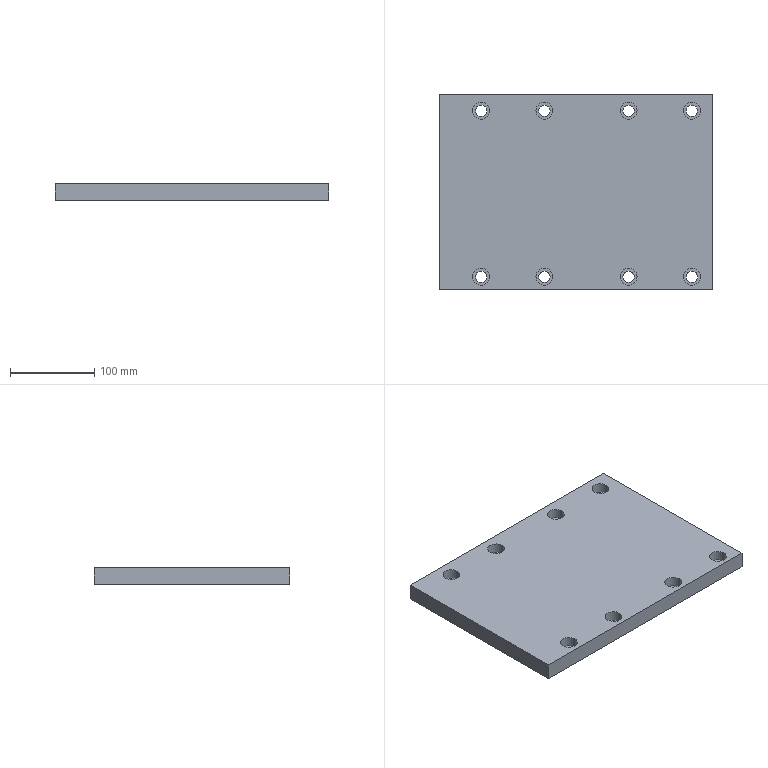Part | SolidWorks | features BaseBody 1 | 1 solid | 46 faces | box 325 x 232 x 20 mm | volume 1468680 mm3 | cylinder 32 | plane 14 | commonest cylinder face diameters 13.5 x16 20 x16
STEP:
#1=CARTESIAN_POINT('',(-122.5,96.448,8.));
#2=VERTEX_POINT('',#1);
#3=CARTESIAN_POINT('',(-102.5,96.448,8.));
#4=VERTEX_POINT('',#3);
#5=CARTESIAN_POINT('',(-112.5,96.448,8.));
#6=DIRECTION('',(0.,0.,1.));
#7=DIRECTION('',(1.,0.,0.));
#8=AXIS2_PLACEMENT_3D('',#5,#6,#7);
#9=CIRCLE('',#8,10.);
#10=EDGE_CURVE('',#2,#4,#9,.T.);
#11=ORIENTED_EDGE('',*,*,#10,.F.);
#12=CARTESIAN_POINT('',(-122.5,96.448,20.));
#13=VERTEX_POINT('',#12);
#14=CARTESIAN_POINT('',(-122.5,96.448,20.));
#15=DIRECTION('',(0.,0.,1.));
#16=VECTOR('',#15,1000.);
#17=LINE('',#14,#16);
#18=EDGE_CURVE('',#2,#13,#17,.T.);
#19=ORIENTED_EDGE('',*,*,#18,.T.);
#20=CARTESIAN_POINT('',(-102.5,96.448,20.));
#21=VERTEX_POINT('',#20);
#22=CARTESIAN_POINT('',(-112.5,96.448,20.));
#23=DIRECTION('',(0.,0.,1.));
#24=DIRECTION('',(1.,0.,0.));
#25=AXIS2_PLACEMENT_3D('',#22,#23,#24);
#26=CIRCLE('',#25,10.);
#27=EDGE_CURVE('',#13,#21,#26,.T.);
#28=ORIENTED_EDGE('',*,*,#27,.T.);
#29=CARTESIAN_POINT('',(-102.5,96.448,20.));
#30=DIRECTION('',(0.,0.,1.));
#31=VECTOR('',#30,1000.);
#32=LINE('',#29,#31);
#33=EDGE_CURVE('',#4,#21,#32,.T.);
#34=ORIENTED_EDGE('',*,*,#33,.F.);
#35=EDGE_LOOP('',(#11,#19,#28,#34));
#36=FACE_OUTER_BOUND('',#35,.T.);
#37=CARTESIAN_POINT('',(-112.5,96.448,20.));
#38=DIRECTION('',(0.,0.,1.));
#39=DIRECTION('',(1.,0.,0.));
#40=AXIS2_PLACEMENT_3D('',#37,#38,#39);
#41=CYLINDRICAL_SURFACE('',#40,10.);
#42=ADVANCED_FACE('',(#36),#41,.F.);
#43=CARTESIAN_POINT('',(-119.25,96.448,0.));
#44=VERTEX_POINT('',#43);
#45=CARTESIAN_POINT('',(-105.75,96.448,0.));
#46=VERTEX_POINT('',#45);
#47=CARTESIAN_POINT('',(-112.5,96.448,0.));
#48=DIRECTION('',(0.,0.,1.));
#49=DIRECTION('',(1.,0.,0.));
#50=AXIS2_PLACEMENT_3D('',#47,#48,#49);
#51=CIRCLE('',#50,6.75);
#52=EDGE_CURVE('',#44,#46,#51,.T.);
#53=ORIENTED_EDGE('',*,*,#52,.F.);
#54=CARTESIAN_POINT('',(-119.25,96.448,8.));
#55=VERTEX_POINT('',#54);
#56=CARTESIAN_POINT('',(-119.25,96.448,20.));
#57=DIRECTION('',(0.,0.,1.));
#58=VECTOR('',#57,1000.);
#59=LINE('',#56,#58);
#60=EDGE_CURVE('',#44,#55,#59,.T.);
#61=ORIENTED_EDGE('',*,*,#60,.T.);
#62=CARTESIAN_POINT('',(-105.75,96.448,8.));
#63=VERTEX_POINT('',#62);
#64=CARTESIAN_POINT('',(-112.5,96.448,8.));
#65=DIRECTION('',(0.,0.,1.));
#66=DIRECTION('',(1.,0.,0.));
#67=AXIS2_PLACEMENT_3D('',#64,#65,#66);
#68=CIRCLE('',#67,6.75);
#69=EDGE_CURVE('',#55,#63,#68,.T.);
#70=ORIENTED_EDGE('',*,*,#69,.T.);
#71=CARTESIAN_POINT('',(-105.75,96.448,20.));
#72=DIRECTION('',(0.,0.,1.));
#73=VECTOR('',#72,1000.);
#74=LINE('',#71,#73);
#75=EDGE_CURVE('',#46,#63,#74,.T.);
#76=ORIENTED_EDGE('',*,*,#75,.F.);
#77=EDGE_LOOP('',(#53,#61,#70,#76));
#78=FACE_OUTER_BOUND('',#77,.T.);
#79=CARTESIAN_POINT('',(-112.5,96.448,20.));
#80=DIRECTION('',(0.,0.,1.));
#81=DIRECTION('',(1.,0.,0.));
#82=AXIS2_PLACEMENT_3D('',#79,#80,#81);
#83=CYLINDRICAL_SURFACE('',#82,6.75);
#84=ADVANCED_FACE('',(#78),#83,.F.);
#85=CARTESIAN_POINT('',(-47.5,96.448,8.));
#86=VERTEX_POINT('',#85);
#87=CARTESIAN_POINT('',(-27.5,96.448,8.));
#88=VERTEX_POINT('',#87);
#89=CARTESIAN_POINT('',(-37.5,96.448,8.));
#90=DIRECTION('',(0.,0.,1.));
#91=DIRECTION('',(1.,0.,0.));
#92=AXIS2_PLACEMENT_3D('',#89,#90,#91);
#93=CIRCLE('',#92,10.);
#94=EDGE_CURVE('',#86,#88,#93,.T.);
#95=ORIENTED_EDGE('',*,*,#94,.F.);
#96=CARTESIAN_POINT('',(-47.5,96.448,20.));
#97=VERTEX_POINT('',#96);
#98=CARTESIAN_POINT('',(-47.5,96.448,20.));
#99=DIRECTION('',(0.,0.,1.));
#100=VECTOR('',#99,1000.);
#101=LINE('',#98,#100);
#102=EDGE_CURVE('',#86,#97,#101,.T.);
#103=ORIENTED_EDGE('',*,*,#102,.T.);
#104=CARTESIAN_POINT('',(-27.5,96.448,20.));
#105=VERTEX_POINT('',#104);
#106=CARTESIAN_POINT('',(-37.5,96.448,20.));
#107=DIRECTION('',(0.,0.,1.));
#108=DIRECTION('',(1.,0.,0.));
#109=AXIS2_PLACEMENT_3D('',#106,#107,#108);
#110=CIRCLE('',#109,10.);
#111=EDGE_CURVE('',#97,#105,#110,.T.);
#112=ORIENTED_EDGE('',*,*,#111,.T.);
#113=CARTESIAN_POINT('',(-27.5,96.448,20.));
#114=DIRECTION('',(0.,0.,1.));
#115=VECTOR('',#114,1000.);
#116=LINE('',#113,#115);
#117=EDGE_CURVE('',#88,#105,#116,.T.);
#118=ORIENTED_EDGE('',*,*,#117,.F.);
#119=EDGE_LOOP('',(#95,#103,#112,#118));
#120=FACE_OUTER_BOUND('',#119,.T.);
#121=CARTESIAN_POINT('',(-37.5,96.448,20.));
#122=DIRECTION('',(0.,0.,1.));
#123=DIRECTION('',(1.,0.,0.));
#124=AXIS2_PLACEMENT_3D('',#121,#122,#123);
#125=CYLINDRICAL_SURFACE('',#124,10.);
#126=ADVANCED_FACE('',(#120),#125,.F.);
#127=CARTESIAN_POINT('',(-44.25,96.448,0.));
#128=VERTEX_POINT('',#127);
#129=CARTESIAN_POINT('',(-30.75,96.448,0.));
#130=VERTEX_POINT('',#129);
#131=CARTESIAN_POINT('',(-37.5,96.448,0.));
#132=DIRECTION('',(0.,0.,1.));
#133=DIRECTION('',(1.,0.,0.));
#134=AXIS2_PLACEMENT_3D('',#131,#132,#133);
#135=CIRCLE('',#134,6.75);
#136=EDGE_CURVE('',#128,#130,#135,.T.);
#137=ORIENTED_EDGE('',*,*,#136,.F.);
#138=CARTESIAN_POINT('',(-44.25,96.448,8.));
#139=VERTEX_POINT('',#138);
#140=CARTESIAN_POINT('',(-44.25,96.448,20.));
#141=DIRECTION('',(0.,0.,1.));
#142=VECTOR('',#141,1000.);
#143=LINE('',#140,#142);
#144=EDGE_CURVE('',#128,#139,#143,.T.);
#145=ORIENTED_EDGE('',*,*,#144,.T.);
#146=CARTESIAN_POINT('',(-30.75,96.448,8.));
#147=VERTEX_POINT('',#146);
#148=CARTESIAN_POINT('',(-37.5,96.448,8.));
#149=DIRECTION('',(0.,0.,1.));
#150=DIRECTION('',(1.,0.,0.));
#151=AXIS2_PLACEMENT_3D('',#148,#149,#150);
#152=CIRCLE('',#151,6.75);
#153=EDGE_CURVE('',#139,#147,#152,.T.);
#154=ORIENTED_EDGE('',*,*,#153,.T.);
#155=CARTESIAN_POINT('',(-30.75,96.448,20.));
#156=DIRECTION('',(0.,0.,1.));
#157=VECTOR('',#156,1000.);
#158=LINE('',#155,#157);
#159=EDGE_CURVE('',#130,#147,#158,.T.);
#160=ORIENTED_EDGE('',*,*,#159,.F.);
#161=EDGE_LOOP('',(#137,#145,#154,#160));
#162=FACE_OUTER_BOUND('',#161,.T.);
#163=CARTESIAN_POINT('',(-37.5,96.448,20.));
#164=DIRECTION('',(0.,0.,1.));
#165=DIRECTION('',(1.,0.,0.));
#166=AXIS2_PLACEMENT_3D('',#163,#164,#165);
#167=CYLINDRICAL_SURFACE('',#166,6.75);
#168=ADVANCED_FACE('',(#162),#167,.F.);
#169=CARTESIAN_POINT('',(52.5,96.448,8.));
#170=VERTEX_POINT('',#169);
#171=CARTESIAN_POINT('',(72.5,96.448,8.));
#172=VERTEX_POINT('',#171);
#173=CARTESIAN_POINT('',(62.5,96.448,8.));
#174=DIRECTION('',(0.,0.,1.));
#175=DIRECTION('',(1.,0.,0.));
#176=AXIS2_PLACEMENT_3D('',#173,#174,#175);
#177=CIRCLE('',#176,10.);
#178=EDGE_CURVE('',#170,#172,#177,.T.);
#179=ORIENTED_EDGE('',*,*,#178,.F.);
#180=CARTESIAN_POINT('',(52.5,96.448,20.));
#181=VERTEX_POINT('',#180);
#182=CARTESIAN_POINT('',(52.5,96.448,20.));
#183=DIRECTION('',(0.,0.,1.));
#184=VECTOR('',#183,1000.);
#185=LINE('',#182,#184);
#186=EDGE_CURVE('',#170,#181,#185,.T.);
#187=ORIENTED_EDGE('',*,*,#186,.T.);
#188=CARTESIAN_POINT('',(72.5,96.448,20.));
#189=VERTEX_POINT('',#188);
#190=CARTESIAN_POINT('',(62.5,96.448,20.));
#191=DIRECTION('',(0.,0.,1.));
#192=DIRECTION('',(1.,0.,0.));
#193=AXIS2_PLACEMENT_3D('',#190,#191,#192);
#194=CIRCLE('',#193,10.);
#195=EDGE_CURVE('',#181,#189,#194,.T.);
#196=ORIENTED_EDGE('',*,*,#195,.T.);
#197=CARTESIAN_POINT('',(72.5,96.448,20.));
#198=DIRECTION('',(0.,0.,1.));
#199=VECTOR('',#198,1000.);
#200=LINE('',#197,#199);
#201=EDGE_CURVE('',#172,#189,#200,.T.);
#202=ORIENTED_EDGE('',*,*,#201,.F.);
#203=EDGE_LOOP('',(#179,#187,#196,#202));
#204=FACE_OUTER_BOUND('',#203,.T.);
#205=CARTESIAN_POINT('',(62.5,96.448,20.));
#206=DIRECTION('',(0.,0.,1.));
#207=DIRECTION('',(1.,0.,0.));
#208=AXIS2_PLACEMENT_3D('',#205,#206,#207);
#209=CYLINDRICAL_SURFACE('',#208,10.);
#210=ADVANCED_FACE('',(#204),#209,.F.);
#211=CARTESIAN_POINT('',(55.75,96.448,0.));
#212=VERTEX_POINT('',#211);
#213=CARTESIAN_POINT('',(69.25,96.448,0.));
#214=VERTEX_POINT('',#213);
#215=CARTESIAN_POINT('',(62.5,96.448,0.));
#216=DIRECTION('',(0.,0.,1.));
#217=DIRECTION('',(1.,0.,0.));
#218=AXIS2_PLACEMENT_3D('',#215,#216,#217);
#219=CIRCLE('',#218,6.75);
#220=EDGE_CURVE('',#212,#214,#219,.T.);
#221=ORIENTED_EDGE('',*,*,#220,.F.);
#222=CARTESIAN_POINT('',(55.75,96.448,8.));
#223=VERTEX_POINT('',#222);
#224=CARTESIAN_POINT('',(55.75,96.448,20.));
#225=DIRECTION('',(0.,0.,1.));
#226=VECTOR('',#225,1000.);
#227=LINE('',#224,#226);
#228=EDGE_CURVE('',#212,#223,#227,.T.);
#229=ORIENTED_EDGE('',*,*,#228,.T.);
#230=CARTESIAN_POINT('',(69.25,96.448,8.));
#231=VERTEX_POINT('',#230);
#232=CARTESIAN_POINT('',(62.5,96.448,8.));
#233=DIRECTION('',(0.,0.,1.));
#234=DIRECTION('',(1.,0.,0.));
#235=AXIS2_PLACEMENT_3D('',#232,#233,#234);
#236=CIRCLE('',#235,6.75);
#237=EDGE_CURVE('',#223,#231,#236,.T.);
#238=ORIENTED_EDGE('',*,*,#237,.T.);
#239=CARTESIAN_POINT('',(69.25,96.448,20.));
#240=DIRECTION('',(0.,0.,1.));
#241=VECTOR('',#240,1000.);
#242=LINE('',#239,#241);
#243=EDGE_CURVE('',#214,#231,#242,.T.);
#244=ORIENTED_EDGE('',*,*,#243,.F.);
#245=EDGE_LOOP('',(#221,#229,#238,#244));
#246=FACE_OUTER_BOUND('',#245,.T.);
#247=CARTESIAN_POINT('',(62.5,96.448,20.));
#248=DIRECTION('',(0.,0.,1.));
#249=DIRECTION('',(1.,0.,0.));
#250=AXIS2_PLACEMENT_3D('',#247,#248,#249);
#251=CYLINDRICAL_SURFACE('',#250,6.75);
#252=ADVANCED_FACE('',(#246),#251,.F.);
#253=CARTESIAN_POINT('',(127.5,96.448,8.));
#254=VERTEX_POINT('',#253);
#255=CARTESIAN_POINT('',(147.5,96.448,8.));
#256=VERTEX_POINT('',#255);
#257=CARTESIAN_POINT('',(137.5,96.448,8.));
#258=DIRECTION('',(0.,0.,1.));
#259=DIRECTION('',(1.,0.,0.));
#260=AXIS2_PLACEMENT_3D('',#257,#258,#259);
#261=CIRCLE('',#260,10.);
#262=EDGE_CURVE('',#254,#256,#261,.T.);
#263=ORIENTED_EDGE('',*,*,#262,.F.);
#264=CARTESIAN_POINT('',(127.5,96.448,20.));
#265=VERTEX_POINT('',#264);
#266=CARTESIAN_POINT('',(127.5,96.448,20.));
#267=DIRECTION('',(0.,0.,1.));
#268=VECTOR('',#267,1000.);
#269=LINE('',#266,#268);
#270=EDGE_CURVE('',#254,#265,#269,.T.);
#271=ORIENTED_EDGE('',*,*,#270,.T.);
#272=CARTESIAN_POINT('',(147.5,96.448,20.));
#273=VERTEX_POINT('',#272);
#274=CARTESIAN_POINT('',(137.5,96.448,20.));
#275=DIRECTION('',(0.,0.,1.));
#276=DIRECTION('',(1.,0.,0.));
#277=AXIS2_PLACEMENT_3D('',#274,#275,#276);
#278=CIRCLE('',#277,10.);
#279=EDGE_CURVE('',#265,#273,#278,.T.);
#280=ORIENTED_EDGE('',*,*,#279,.T.);
#281=CARTESIAN_POINT('',(147.5,96.448,20.));
#282=DIRECTION('',(0.,0.,1.));
#283=VECTOR('',#282,1000.);
#284=LINE('',#281,#283);
#285=EDGE_CURVE('',#256,#273,#284,.T.);
#286=ORIENTED_EDGE('',*,*,#285,.F.);
#287=EDGE_LOOP('',(#263,#271,#280,#286));
#288=FACE_OUTER_BOUND('',#287,.T.);
#289=CARTESIAN_POINT('',(137.5,96.448,20.));
#290=DIRECTION('',(0.,0.,1.));
#291=DIRECTION('',(1.,0.,0.));
#292=AXIS2_PLACEMENT_3D('',#289,#290,#291);
#293=CYLINDRICAL_SURFACE('',#292,10.);
#294=ADVANCED_FACE('',(#288),#293,.F.);
#295=CARTESIAN_POINT('',(130.75,96.448,0.));
#296=VERTEX_POINT('',#295);
#297=CARTESIAN_POINT('',(144.25,96.448,0.));
#298=VERTEX_POINT('',#297);
#299=CARTESIAN_POINT('',(137.5,96.448,0.));
#300=DIRECTION('',(0.,0.,1.));
#301=DIRECTION('',(1.,0.,0.));
#302=AXIS2_PLACEMENT_3D('',#299,#300,#301);
#303=CIRCLE('',#302,6.75);
#304=EDGE_CURVE('',#296,#298,#303,.T.);
#305=ORIENTED_EDGE('',*,*,#304,.F.);
#306=CARTESIAN_POINT('',(130.75,96.448,8.));
#307=VERTEX_POINT('',#306);
#308=CARTESIAN_POINT('',(130.75,96.448,20.));
#309=DIRECTION('',(0.,0.,1.));
#310=VECTOR('',#309,1000.);
#311=LINE('',#308,#310);
#312=EDGE_CURVE('',#296,#307,#311,.T.);
#313=ORIENTED_EDGE('',*,*,#312,.T.);
#314=CARTESIAN_POINT('',(144.25,96.448,8.));
#315=VERTEX_POINT('',#314);
#316=CARTESIAN_POINT('',(137.5,96.448,8.));
#317=DIRECTION('',(0.,0.,1.));
#318=DIRECTION('',(1.,0.,0.));
#319=AXIS2_PLACEMENT_3D('',#316,#317,#318);
#320=CIRCLE('',#319,6.75);
#321=EDGE_CURVE('',#307,#315,#320,.T.);
#322=ORIENTED_EDGE('',*,*,#321,.T.);
#323=CARTESIAN_POINT('',(144.25,96.448,20.));
#324=DIRECTION('',(0.,0.,1.));
#325=VECTOR('',#324,1000.);
#326=LINE('',#323,#325);
#327=EDGE_CURVE('',#298,#315,#326,.T.);
#328=ORIENTED_EDGE('',*,*,#327,.F.);
#329=EDGE_LOOP('',(#305,#313,#322,#328));
#330=FACE_OUTER_BOUND('',#329,.T.);
#331=CARTESIAN_POINT('',(137.5,96.448,20.));
#332=DIRECTION('',(0.,0.,1.));
#333=DIRECTION('',(1.,0.,0.));
#334=AXIS2_PLACEMENT_3D('',#331,#332,#333);
#335=CYLINDRICAL_SURFACE('',#334,6.75);
#336=ADVANCED_FACE('',(#330),#335,.F.);
#337=CARTESIAN_POINT('',(127.5,-100.552,8.));
#338=VERTEX_POINT('',#337);
#339=CARTESIAN_POINT('',(147.5,-100.552,8.));
#340=VERTEX_POINT('',#339);
#341=CARTESIAN_POINT('',(137.5,-100.552,8.));
#342=DIRECTION('',(0.,0.,1.));
#343=DIRECTION('',(1.,0.,0.));
#344=AXIS2_PLACEMENT_3D('',#341,#342,#343);
#345=CIRCLE('',#344,10.);
#346=EDGE_CURVE('',#338,#340,#345,.T.);
#347=ORIENTED_EDGE('',*,*,#346,.F.);
#348=CARTESIAN_POINT('',(127.5,-100.552,20.));
#349=VERTEX_POINT('',#348);
#350=CARTESIAN_POINT('',(127.5,-100.552,20.));
#351=DIRECTION('',(0.,0.,1.));
#352=VECTOR('',#351,1000.);
#353=LINE('',#350,#352);
#354=EDGE_CURVE('',#338,#349,#353,.T.);
#355=ORIENTED_EDGE('',*,*,#354,.T.);
#356=CARTESIAN_POINT('',(147.5,-100.552,20.));
#357=VERTEX_POINT('',#356);
#358=CARTESIAN_POINT('',(137.5,-100.552,20.));
#359=DIRECTION('',(0.,0.,1.));
#360=DIRECTION('',(1.,0.,0.));
#361=AXIS2_PLACEMENT_3D('',#358,#359,#360);
#362=CIRCLE('',#361,10.);
#363=EDGE_CURVE('',#349,#357,#362,.T.);
#364=ORIENTED_EDGE('',*,*,#363,.T.);
#365=CARTESIAN_POINT('',(147.5,-100.552,20.));
#366=DIRECTION('',(0.,0.,1.));
#367=VECTOR('',#366,1000.);
#368=LINE('',#365,#367);
#369=EDGE_CURVE('',#340,#357,#368,.T.);
#370=ORIENTED_EDGE('',*,*,#369,.F.);
#371=EDGE_LOOP('',(#347,#355,#364,#370));
#372=FACE_OUTER_BOUND('',#371,.T.);
#373=CARTESIAN_POINT('',(137.5,-100.552,20.));
#374=DIRECTION('',(0.,0.,1.));
#375=DIRECTION('',(1.,0.,0.));
#376=AXIS2_PLACEMENT_3D('',#373,#374,#375);
#377=CYLINDRICAL_SURFACE('',#376,10.);
#378=ADVANCED_FACE('',(#372),#377,.F.);
#379=CARTESIAN_POINT('',(130.75,-100.552,0.));
#380=VERTEX_POINT('',#379);
#381=CARTESIAN_POINT('',(144.25,-100.552,0.));
#382=VERTEX_POINT('',#381);
#383=CARTESIAN_POINT('',(137.5,-100.552,0.));
#384=DIRECTION('',(0.,0.,1.));
#385=DIRECTION('',(1.,0.,0.));
#386=AXIS2_PLACEMENT_3D('',#383,#384,#385);
#387=CIRCLE('',#386,6.75);
#388=EDGE_CURVE('',#380,#382,#387,.T.);
#389=ORIENTED_EDGE('',*,*,#388,.F.);
#390=CARTESIAN_POINT('',(130.75,-100.552,8.));
#391=VERTEX_POINT('',#390);
#392=CARTESIAN_POINT('',(130.75,-100.552,20.));
#393=DIRECTION('',(0.,0.,1.));
#394=VECTOR('',#393,1000.);
#395=LINE('',#392,#394);
#396=EDGE_CURVE('',#380,#391,#395,.T.);
#397=ORIENTED_EDGE('',*,*,#396,.T.);
#398=CARTESIAN_POINT('',(144.25,-100.552,8.));
#399=VERTEX_POINT('',#398);
#400=CARTESIAN_POINT('',(137.5,-100.552,8.));
#401=DIRECTION('',(0.,0.,1.));
#402=DIRECTION('',(1.,0.,0.));
#403=AXIS2_PLACEMENT_3D('',#400,#401,#402);
#404=CIRCLE('',#403,6.75);
#405=EDGE_CURVE('',#391,#399,#404,.T.);
#406=ORIENTED_EDGE('',*,*,#405,.T.);
#407=CARTESIAN_POINT('',(144.25,-100.552,20.));
#408=DIRECTION('',(0.,0.,1.));
#409=VECTOR('',#408,1000.);
#410=LINE('',#407,#409);
#411=EDGE_CURVE('',#382,#399,#410,.T.);
#412=ORIENTED_EDGE('',*,*,#411,.F.);
#413=EDGE_LOOP('',(#389,#397,#406,#412));
#414=FACE_OUTER_BOUND('',#413,.T.);
#415=CARTESIAN_POINT('',(137.5,-100.552,20.));
#416=DIRECTION('',(0.,0.,1.));
#417=DIRECTION('',(1.,0.,0.));
#418=AXIS2_PLACEMENT_3D('',#415,#416,#417);
#419=CYLINDRICAL_SURFACE('',#418,6.75);
#420=ADVANCED_FACE('',(#414),#419,.F.);
#421=CARTESIAN_POINT('',(52.5,-100.552,8.));
#422=VERTEX_POINT('',#421);
#423=CARTESIAN_POINT('',(72.5,-100.552,8.));
#424=VERTEX_POINT('',#423);
#425=CARTESIAN_POINT('',(62.5,-100.552,8.));
#426=DIRECTION('',(0.,0.,1.));
#427=DIRECTION('',(1.,0.,0.));
#428=AXIS2_PLACEMENT_3D('',#425,#426,#427);
#429=CIRCLE('',#428,10.);
#430=EDGE_CURVE('',#422,#424,#429,.T.);
#431=ORIENTED_EDGE('',*,*,#430,.F.);
#432=CARTESIAN_POINT('',(52.5,-100.552,20.));
#433=VERTEX_POINT('',#432);
#434=CARTESIAN_POINT('',(52.5,-100.552,20.));
#435=DIRECTION('',(0.,0.,1.));
#436=VECTOR('',#435,1000.);
#437=LINE('',#434,#436);
#438=EDGE_CURVE('',#422,#433,#437,.T.);
#439=ORIENTED_EDGE('',*,*,#438,.T.);
#440=CARTESIAN_POINT('',(72.5,-100.552,20.));
#441=VERTEX_POINT('',#440);
#442=CARTESIAN_POINT('',(62.5,-100.552,20.));
#443=DIRECTION('',(0.,0.,1.));
#444=DIRECTION('',(1.,0.,0.));
#445=AXIS2_PLACEMENT_3D('',#442,#443,#444);
#446=CIRCLE('',#445,10.);
#447=EDGE_CURVE('',#433,#441,#446,.T.);
#448=ORIENTED_EDGE('',*,*,#447,.T.);
#449=CARTESIAN_POINT('',(72.5,-100.552,20.));
#450=DIRECTION('',(0.,0.,1.));
#451=VECTOR('',#450,1000.);
#452=LINE('',#449,#451);
#453=EDGE_CURVE('',#424,#441,#452,.T.);
#454=ORIENTED_EDGE('',*,*,#453,.F.);
#455=EDGE_LOOP('',(#431,#439,#448,#454));
#456=FACE_OUTER_BOUND('',#455,.T.);
#457=CARTESIAN_POINT('',(62.5,-100.552,20.));
#458=DIRECTION('',(0.,0.,1.));
#459=DIRECTION('',(1.,0.,0.));
#460=AXIS2_PLACEMENT_3D('',#457,#458,#459);
#461=CYLINDRICAL_SURFACE('',#460,10.);
#462=ADVANCED_FACE('',(#456),#461,.F.);
#463=CARTESIAN_POINT('',(55.75,-100.552,0.));
#464=VERTEX_POINT('',#463);
#465=CARTESIAN_POINT('',(69.25,-100.552,0.));
#466=VERTEX_POINT('',#465);
#467=CARTESIAN_POINT('',(62.5,-100.552,0.));
#468=DIRECTION('',(0.,0.,1.));
#469=DIRECTION('',(1.,0.,0.));
#470=AXIS2_PLACEMENT_3D('',#467,#468,#469);
#471=CIRCLE('',#470,6.75);
#472=EDGE_CURVE('',#464,#466,#471,.T.);
#473=ORIENTED_EDGE('',*,*,#472,.F.);
#474=CARTESIAN_POINT('',(55.75,-100.552,8.));
#475=VERTEX_POINT('',#474);
#476=CARTESIAN_POINT('',(55.75,-100.552,20.));
#477=DIRECTION('',(0.,0.,1.));
#478=VECTOR('',#477,1000.);
#479=LINE('',#476,#478);
#480=EDGE_CURVE('',#464,#475,#479,.T.);
#481=ORIENTED_EDGE('',*,*,#480,.T.);
#482=CARTESIAN_POINT('',(69.25,-100.552,8.));
#483=VERTEX_POINT('',#482);
#484=CARTESIAN_POINT('',(62.5,-100.552,8.));
#485=DIRECTION('',(0.,0.,1.));
#486=DIRECTION('',(1.,0.,0.));
#487=AXIS2_PLACEMENT_3D('',#484,#485,#486);
#488=CIRCLE('',#487,6.75);
#489=EDGE_CURVE('',#475,#483,#488,.T.);
#490=ORIENTED_EDGE('',*,*,#489,.T.);
#491=CARTESIAN_POINT('',(69.25,-100.552,20.));
#492=DIRECTION('',(0.,0.,1.));
#493=VECTOR('',#492,1000.);
#494=LINE('',#491,#493);
#495=EDGE_CURVE('',#466,#483,#494,.T.);
#496=ORIENTED_EDGE('',*,*,#495,.F.);
#497=EDGE_LOOP('',(#473,#481,#490,#496));
#498=FACE_OUTER_BOUND('',#497,.T.);
#499=CARTESIAN_POINT('',(62.5,-100.552,20.));
#500=DIRECTION('',(0.,0.,1.));
#501=DIRECTION('',(1.,0.,0.));
#502=AXIS2_PLACEMENT_3D('',#499,#500,#501);
#503=CYLINDRICAL_SURFACE('',#502,6.75);
#504=ADVANCED_FACE('',(#498),#503,.F.);
#505=CARTESIAN_POINT('',(-47.5,-100.552,8.));
#506=VERTEX_POINT('',#505);
#507=CARTESIAN_POINT('',(-27.5,-100.552,8.));
#508=VERTEX_POINT('',#507);
#509=CARTESIAN_POINT('',(-37.5,-100.552,8.));
#510=DIRECTION('',(0.,0.,1.));
#511=DIRECTION('',(1.,0.,0.));
#512=AXIS2_PLACEMENT_3D('',#509,#510,#511);
#513=CIRCLE('',#512,10.);
#514=EDGE_CURVE('',#506,#508,#513,.T.);
#515=ORIENTED_EDGE('',*,*,#514,.F.);
#516=CARTESIAN_POINT('',(-47.5,-100.552,20.));
#517=VERTEX_POINT('',#516);
#518=CARTESIAN_POINT('',(-47.5,-100.552,20.));
#519=DIRECTION('',(0.,0.,1.));
#520=VECTOR('',#519,1000.);
#521=LINE('',#518,#520);
#522=EDGE_CURVE('',#506,#517,#521,.T.);
#523=ORIENTED_EDGE('',*,*,#522,.T.);
#524=CARTESIAN_POINT('',(-27.5,-100.552,20.));
#525=VERTEX_POINT('',#524);
#526=CARTESIAN_POINT('',(-37.5,-100.552,20.));
#527=DIRECTION('',(0.,0.,1.));
#528=DIRECTION('',(1.,0.,0.));
#529=AXIS2_PLACEMENT_3D('',#526,#527,#528);
#530=CIRCLE('',#529,10.);
#531=EDGE_CURVE('',#517,#525,#530,.T.);
#532=ORIENTED_EDGE('',*,*,#531,.T.);
#533=CARTESIAN_POINT('',(-27.5,-100.552,20.));
#534=DIRECTION('',(0.,0.,1.));
#535=VECTOR('',#534,1000.);
#536=LINE('',#533,#535);
#537=EDGE_CURVE('',#508,#525,#536,.T.);
#538=ORIENTED_EDGE('',*,*,#537,.F.);
#539=EDGE_LOOP('',(#515,#523,#532,#538));
#540=FACE_OUTER_BOUND('',#539,.T.);
#541=CARTESIAN_POINT('',(-37.5,-100.552,20.));
#542=DIRECTION('',(0.,0.,1.));
#543=DIRECTION('',(1.,0.,0.));
#544=AXIS2_PLACEMENT_3D('',#541,#542,#543);
#545=CYLINDRICAL_SURFACE('',#544,10.);
#546=ADVANCED_FACE('',(#540),#545,.F.);
#547=CARTESIAN_POINT('',(-44.25,-100.552,0.));
#548=VERTEX_POINT('',#547);
#549=CARTESIAN_POINT('',(-30.75,-100.552,0.));
#550=VERTEX_POINT('',#549);
#551=CARTESIAN_POINT('',(-37.5,-100.552,0.));
#552=DIRECTION('',(0.,0.,1.));
#553=DIRECTION('',(1.,0.,0.));
#554=AXIS2_PLACEMENT_3D('',#551,#552,#553);
#555=CIRCLE('',#554,6.75);
#556=EDGE_CURVE('',#548,#550,#555,.T.);
#557=ORIENTED_EDGE('',*,*,#556,.F.);
#558=CARTESIAN_POINT('',(-44.25,-100.552,8.));
#559=VERTEX_POINT('',#558);
#560=CARTESIAN_POINT('',(-44.25,-100.552,20.));
#561=DIRECTION('',(0.,0.,1.));
#562=VECTOR('',#561,1000.);
#563=LINE('',#560,#562);
#564=EDGE_CURVE('',#548,#559,#563,.T.);
#565=ORIENTED_EDGE('',*,*,#564,.T.);
#566=CARTESIAN_POINT('',(-30.75,-100.552,8.));
#567=VERTEX_POINT('',#566);
#568=CARTESIAN_POINT('',(-37.5,-100.552,8.));
#569=DIRECTION('',(0.,0.,1.));
#570=DIRECTION('',(1.,0.,0.));
#571=AXIS2_PLACEMENT_3D('',#568,#569,#570);
#572=CIRCLE('',#571,6.75);
#573=EDGE_CURVE('',#559,#567,#572,.T.);
#574=ORIENTED_EDGE('',*,*,#573,.T.);
#575=CARTESIAN_POINT('',(-30.75,-100.552,20.));
#576=DIRECTION('',(0.,0.,1.));
#577=VECTOR('',#576,1000.);
#578=LINE('',#575,#577);
#579=EDGE_CURVE('',#550,#567,#578,.T.);
#580=ORIENTED_EDGE('',*,*,#579,.F.);
#581=EDGE_LOOP('',(#557,#565,#574,#580));
#582=FACE_OUTER_BOUND('',#581,.T.);
#583=CARTESIAN_POINT('',(-37.5,-100.552,20.));
#584=DIRECTION('',(0.,0.,1.));
#585=DIRECTION('',(1.,0.,0.));
#586=AXIS2_PLACEMENT_3D('',#583,#584,#585);
#587=CYLINDRICAL_SURFACE('',#586,6.75);
#588=ADVANCED_FACE('',(#582),#587,.F.);
#589=CARTESIAN_POINT('',(-122.5,-100.552,8.));
#590=VERTEX_POINT('',#589);
#591=CARTESIAN_POINT('',(-102.5,-100.552,8.));
#592=VERTEX_POINT('',#591);
#593=CARTESIAN_POINT('',(-112.5,-100.552,8.));
#594=DIRECTION('',(0.,0.,1.));
#595=DIRECTION('',(1.,0.,0.));
#596=AXIS2_PLACEMENT_3D('',#593,#594,#595);
#597=CIRCLE('',#596,10.);
#598=EDGE_CURVE('',#590,#592,#597,.T.);
#599=ORIENTED_EDGE('',*,*,#598,.F.);
#600=CARTESIAN_POINT('',(-122.5,-100.552,20.));
#601=VERTEX_POINT('',#600);
#602=CARTESIAN_POINT('',(-122.5,-100.552,20.));
#603=DIRECTION('',(0.,0.,1.));
#604=VECTOR('',#603,1000.);
#605=LINE('',#602,#604);
#606=EDGE_CURVE('',#590,#601,#605,.T.);
#607=ORIENTED_EDGE('',*,*,#606,.T.);
#608=CARTESIAN_POINT('',(-102.5,-100.552,20.));
#609=VERTEX_POINT('',#608);
#610=CARTESIAN_POINT('',(-112.5,-100.552,20.));
#611=DIRECTION('',(0.,0.,1.));
#612=DIRECTION('',(1.,0.,0.));
#613=AXIS2_PLACEMENT_3D('',#610,#611,#612);
#614=CIRCLE('',#613,10.);
#615=EDGE_CURVE('',#601,#609,#614,.T.);
#616=ORIENTED_EDGE('',*,*,#615,.T.);
#617=CARTESIAN_POINT('',(-102.5,-100.552,20.));
#618=DIRECTION('',(0.,0.,1.));
#619=VECTOR('',#618,1000.);
#620=LINE('',#617,#619);
#621=EDGE_CURVE('',#592,#609,#620,.T.);
#622=ORIENTED_EDGE('',*,*,#621,.F.);
#623=EDGE_LOOP('',(#599,#607,#616,#622));
#624=FACE_OUTER_BOUND('',#623,.T.);
#625=CARTESIAN_POINT('',(-112.5,-100.552,20.));
#626=DIRECTION('',(0.,0.,1.));
#627=DIRECTION('',(1.,0.,0.));
#628=AXIS2_PLACEMENT_3D('',#625,#626,#627);
#629=CYLINDRICAL_SURFACE('',#628,10.);
#630=ADVANCED_FACE('',(#624),#629,.F.);
#631=CARTESIAN_POINT('',(-119.25,-100.552,0.));
#632=VERTEX_POINT('',#631);
#633=CARTESIAN_POINT('',(-105.75,-100.552,0.));
#634=VERTEX_POINT('',#633);
#635=CARTESIAN_POINT('',(-112.5,-100.552,0.));
#636=DIRECTION('',(0.,0.,1.));
#637=DIRECTION('',(1.,0.,0.));
#638=AXIS2_PLACEMENT_3D('',#635,#636,#637);
#639=CIRCLE('',#638,6.75);
#640=EDGE_CURVE('',#632,#634,#639,.T.);
#641=ORIENTED_EDGE('',*,*,#640,.F.);
#642=CARTESIAN_POINT('',(-119.25,-100.552,8.));
#643=VERTEX_POINT('',#642);
#644=CARTESIAN_POINT('',(-119.25,-100.552,20.));
#645=DIRECTION('',(0.,0.,1.));
#646=VECTOR('',#645,1000.);
#647=LINE('',#644,#646);
#648=EDGE_CURVE('',#632,#643,#647,.T.);
#649=ORIENTED_EDGE('',*,*,#648,.T.);
#650=CARTESIAN_POINT('',(-105.75,-100.552,8.));
#651=VERTEX_POINT('',#650);
#652=CARTESIAN_POINT('',(-112.5,-100.552,8.));
#653=DIRECTION('',(0.,0.,1.));
#654=DIRECTION('',(1.,0.,0.));
#655=AXIS2_PLACEMENT_3D('',#652,#653,#654);
#656=CIRCLE('',#655,6.75);
#657=EDGE_CURVE('',#643,#651,#656,.T.);
#658=ORIENTED_EDGE('',*,*,#657,.T.);
#659=CARTESIAN_POINT('',(-105.75,-100.552,20.));
#660=DIRECTION('',(0.,0.,1.));
#661=VECTOR('',#660,1000.);
#662=LINE('',#659,#661);
#663=EDGE_CURVE('',#634,#651,#662,.T.);
#664=ORIENTED_EDGE('',*,*,#663,.F.);
#665=EDGE_LOOP('',(#641,#649,#658,#664));
#666=FACE_OUTER_BOUND('',#665,.T.);
#667=CARTESIAN_POINT('',(-112.5,-100.552,20.));
#668=DIRECTION('',(0.,0.,1.));
#669=DIRECTION('',(1.,0.,0.));
#670=AXIS2_PLACEMENT_3D('',#667,#668,#669);
#671=CYLINDRICAL_SURFACE('',#670,6.75);
#672=ADVANCED_FACE('',(#666),#671,.F.);
#673=CARTESIAN_POINT('',(-162.5,116.,0.));
#674=VERTEX_POINT('',#673);
#675=CARTESIAN_POINT('',(-162.5,-116.,0.));
#676=VERTEX_POINT('',#675);
#677=CARTESIAN_POINT('',(-162.5,-116.,0.));
#678=DIRECTION('',(0.,-1.,0.));
#679=VECTOR('',#678,1000.);
#680=LINE('',#677,#679);
#681=EDGE_CURVE('',#674,#676,#680,.T.);
#682=ORIENTED_EDGE('',*,*,#681,.T.);
#683=CARTESIAN_POINT('',(-162.5,-116.,20.));
#684=VERTEX_POINT('',#683);
#685=CARTESIAN_POINT('',(-162.5,-116.,20.));
#686=DIRECTION('',(0.,0.,-1.));
#687=VECTOR('',#686,1000.);
#688=LINE('',#685,#687);
#689=EDGE_CURVE('',#684,#676,#688,.T.);
#690=ORIENTED_EDGE('',*,*,#689,.F.);
#691=CARTESIAN_POINT('',(-162.5,116.,20.));
#692=VERTEX_POINT('',#691);
#693=CARTESIAN_POINT('',(-162.5,-116.,20.));
#694=DIRECTION('',(0.,-1.,0.));
#695=VECTOR('',#694,1000.);
#696=LINE('',#693,#695);
#697=EDGE_CURVE('',#692,#684,#696,.T.);
#698=ORIENTED_EDGE('',*,*,#697,.F.);
#699=CARTESIAN_POINT('',(-162.5,116.,20.));
#700=DIRECTION('',(0.,0.,-1.));
#701=VECTOR('',#700,1000.);
#702=LINE('',#699,#701);
#703=EDGE_CURVE('',#692,#674,#702,.T.);
#704=ORIENTED_EDGE('',*,*,#703,.T.);
#705=EDGE_LOOP('',(#682,#690,#698,#704));
#706=FACE_OUTER_BOUND('',#705,.T.);
#707=CARTESIAN_POINT('',(-162.5,-116.,20.));
#708=DIRECTION('',(1.,0.,0.));
#709=DIRECTION('',(0.,0.,-1.));
#710=AXIS2_PLACEMENT_3D('',#707,#708,#709);
#711=PLANE('',#710);
#712=ADVANCED_FACE('',(#706),#711,.F.);
#713=CARTESIAN_POINT('',(162.5,-116.,0.));
#714=VERTEX_POINT('',#713);
#715=CARTESIAN_POINT('',(162.5,-116.,0.));
#716=DIRECTION('',(1.,0.,0.));
#717=VECTOR('',#716,1000.);
#718=LINE('',#715,#717);
#719=EDGE_CURVE('',#676,#714,#718,.T.);
#720=ORIENTED_EDGE('',*,*,#719,.T.);
#721=CARTESIAN_POINT('',(162.5,-116.,20.));
#722=VERTEX_POINT('',#721);
#723=CARTESIAN_POINT('',(162.5,-116.,20.));
#724=DIRECTION('',(0.,0.,-1.));
#725=VECTOR('',#724,1000.);
#726=LINE('',#723,#725);
#727=EDGE_CURVE('',#722,#714,#726,.T.);
#728=ORIENTED_EDGE('',*,*,#727,.F.);
#729=CARTESIAN_POINT('',(162.5,-116.,20.));
#730=DIRECTION('',(1.,0.,0.));
#731=VECTOR('',#730,1000.);
#732=LINE('',#729,#731);
#733=EDGE_CURVE('',#684,#722,#732,.T.);
#734=ORIENTED_EDGE('',*,*,#733,.F.);
#735=ORIENTED_EDGE('',*,*,#689,.T.);
#736=EDGE_LOOP('',(#720,#728,#734,#735));
#737=FACE_OUTER_BOUND('',#736,.T.);
#738=CARTESIAN_POINT('',(162.5,-116.,20.));
#739=DIRECTION('',(0.,1.,0.));
#740=DIRECTION('',(-1.,0.,0.));
#741=AXIS2_PLACEMENT_3D('',#738,#739,#740);
#742=PLANE('',#741);
#743=ADVANCED_FACE('',(#737),#742,.F.);
#744=CARTESIAN_POINT('',(162.5,116.,0.));
#745=VERTEX_POINT('',#744);
#746=CARTESIAN_POINT('',(162.5,-116.,0.));
#747=DIRECTION('',(0.,1.,0.));
#748=VECTOR('',#747,1000.);
#749=LINE('',#746,#748);
#750=EDGE_CURVE('',#714,#745,#749,.T.);
#751=ORIENTED_EDGE('',*,*,#750,.T.);
#752=CARTESIAN_POINT('',(162.5,116.,20.));
#753=VERTEX_POINT('',#752);
#754=CARTESIAN_POINT('',(162.5,116.,20.));
#755=DIRECTION('',(0.,0.,-1.));
#756=VECTOR('',#755,1000.);
#757=LINE('',#754,#756);
#758=EDGE_CURVE('',#753,#745,#757,.T.);
#759=ORIENTED_EDGE('',*,*,#758,.F.);
#760=CARTESIAN_POINT('',(162.5,-116.,20.));
#761=DIRECTION('',(0.,1.,0.));
#762=VECTOR('',#761,1000.);
#763=LINE('',#760,#762);
#764=EDGE_CURVE('',#722,#753,#763,.T.);
#765=ORIENTED_EDGE('',*,*,#764,.F.);
#766=ORIENTED_EDGE('',*,*,#727,.T.);
#767=EDGE_LOOP('',(#751,#759,#765,#766));
#768=FACE_OUTER_BOUND('',#767,.T.);
#769=CARTESIAN_POINT('',(162.5,-116.,20.));
#770=DIRECTION('',(-1.,0.,0.));
#771=DIRECTION('',(0.,0.,1.));
#772=AXIS2_PLACEMENT_3D('',#769,#770,#771);
#773=PLANE('',#772);
#774=ADVANCED_FACE('',(#768),#773,.F.);
#775=CARTESIAN_POINT('',(162.5,116.,0.));
#776=DIRECTION('',(-1.,0.,0.));
#777=VECTOR('',#776,1000.);
#778=LINE('',#775,#777);
#779=EDGE_CURVE('',#745,#674,#778,.T.);
#780=ORIENTED_EDGE('',*,*,#779,.T.);
#781=ORIENTED_EDGE('',*,*,#703,.F.);
#782=CARTESIAN_POINT('',(162.5,116.,20.));
#783=DIRECTION('',(-1.,0.,0.));
#784=VECTOR('',#783,1000.);
#785=LINE('',#782,#784);
#786=EDGE_CURVE('',#753,#692,#785,.T.);
#787=ORIENTED_EDGE('',*,*,#786,.F.);
#788=ORIENTED_EDGE('',*,*,#758,.T.);
#789=EDGE_LOOP('',(#780,#781,#787,#788));
#790=FACE_OUTER_BOUND('',#789,.T.);
#791=CARTESIAN_POINT('',(162.5,116.,20.));
#792=DIRECTION('',(0.,-1.,0.));
#793=DIRECTION('',(1.,0.,0.));
#794=AXIS2_PLACEMENT_3D('',#791,#792,#793);
#795=PLANE('',#794);
#796=ADVANCED_FACE('',(#790),#795,.F.);
#797=CARTESIAN_POINT('',(-112.5,96.448,20.));
#798=DIRECTION('',(0.,0.,1.));
#799=DIRECTION('',(1.,0.,0.));
#800=AXIS2_PLACEMENT_3D('',#797,#798,#799);
#801=CIRCLE('',#800,10.);
#802=EDGE_CURVE('',#21,#13,#801,.T.);
#803=ORIENTED_EDGE('',*,*,#802,.F.);
#804=ORIENTED_EDGE('',*,*,#27,.F.);
#805=EDGE_LOOP('',(#803,#804));
#806=FACE_BOUND('',#805,.T.);
#807=CARTESIAN_POINT('',(-37.5,96.448,20.));
#808=DIRECTION('',(0.,0.,1.));
#809=DIRECTION('',(1.,0.,0.));
#810=AXIS2_PLACEMENT_3D('',#807,#808,#809);
#811=CIRCLE('',#810,10.);
#812=EDGE_CURVE('',#105,#97,#811,.T.);
#813=ORIENTED_EDGE('',*,*,#812,.F.);
#814=ORIENTED_EDGE('',*,*,#111,.F.);
#815=EDGE_LOOP('',(#813,#814));
#816=FACE_BOUND('',#815,.T.);
#817=CARTESIAN_POINT('',(62.5,96.448,20.));
#818=DIRECTION('',(0.,0.,1.));
#819=DIRECTION('',(1.,0.,0.));
#820=AXIS2_PLACEMENT_3D('',#817,#818,#819);
#821=CIRCLE('',#820,10.);
#822=EDGE_CURVE('',#189,#181,#821,.T.);
#823=ORIENTED_EDGE('',*,*,#822,.F.);
#824=ORIENTED_EDGE('',*,*,#195,.F.);
#825=EDGE_LOOP('',(#823,#824));
#826=FACE_BOUND('',#825,.T.);
#827=CARTESIAN_POINT('',(137.5,96.448,20.));
#828=DIRECTION('',(0.,0.,1.));
#829=DIRECTION('',(1.,0.,0.));
#830=AXIS2_PLACEMENT_3D('',#827,#828,#829);
#831=CIRCLE('',#830,10.);
#832=EDGE_CURVE('',#273,#265,#831,.T.);
#833=ORIENTED_EDGE('',*,*,#832,.F.);
#834=ORIENTED_EDGE('',*,*,#279,.F.);
#835=EDGE_LOOP('',(#833,#834));
#836=FACE_BOUND('',#835,.T.);
#837=CARTESIAN_POINT('',(137.5,-100.552,20.));
#838=DIRECTION('',(0.,0.,1.));
#839=DIRECTION('',(1.,0.,0.));
#840=AXIS2_PLACEMENT_3D('',#837,#838,#839);
#841=CIRCLE('',#840,10.);
#842=EDGE_CURVE('',#357,#349,#841,.T.);
#843=ORIENTED_EDGE('',*,*,#842,.F.);
#844=ORIENTED_EDGE('',*,*,#363,.F.);
#845=EDGE_LOOP('',(#843,#844));
#846=FACE_BOUND('',#845,.T.);
#847=CARTESIAN_POINT('',(62.5,-100.552,20.));
#848=DIRECTION('',(0.,0.,1.));
#849=DIRECTION('',(1.,0.,0.));
#850=AXIS2_PLACEMENT_3D('',#847,#848,#849);
#851=CIRCLE('',#850,10.);
#852=EDGE_CURVE('',#441,#433,#851,.T.);
#853=ORIENTED_EDGE('',*,*,#852,.F.);
#854=ORIENTED_EDGE('',*,*,#447,.F.);
#855=EDGE_LOOP('',(#853,#854));
#856=FACE_BOUND('',#855,.T.);
#857=CARTESIAN_POINT('',(-37.5,-100.552,20.));
#858=DIRECTION('',(0.,0.,1.));
#859=DIRECTION('',(1.,0.,0.));
#860=AXIS2_PLACEMENT_3D('',#857,#858,#859);
#861=CIRCLE('',#860,10.);
#862=EDGE_CURVE('',#525,#517,#861,.T.);
#863=ORIENTED_EDGE('',*,*,#862,.F.);
#864=ORIENTED_EDGE('',*,*,#531,.F.);
#865=EDGE_LOOP('',(#863,#864));
#866=FACE_BOUND('',#865,.T.);
#867=CARTESIAN_POINT('',(-112.5,-100.552,20.));
#868=DIRECTION('',(0.,0.,1.));
#869=DIRECTION('',(1.,0.,0.));
#870=AXIS2_PLACEMENT_3D('',#867,#868,#869);
#871=CIRCLE('',#870,10.);
#872=EDGE_CURVE('',#609,#601,#871,.T.);
#873=ORIENTED_EDGE('',*,*,#872,.F.);
#874=ORIENTED_EDGE('',*,*,#615,.F.);
#875=EDGE_LOOP('',(#873,#874));
#876=FACE_BOUND('',#875,.T.);
#877=ORIENTED_EDGE('',*,*,#697,.T.);
#878=ORIENTED_EDGE('',*,*,#733,.T.);
#879=ORIENTED_EDGE('',*,*,#764,.T.);
#880=ORIENTED_EDGE('',*,*,#786,.T.);
#881=EDGE_LOOP('',(#877,#878,#879,#880));
#882=FACE_OUTER_BOUND('',#881,.T.);
#883=CARTESIAN_POINT('',(0.,0.,20.));
#884=DIRECTION('',(0.,0.,1.));
#885=DIRECTION('',(1.,0.,0.));
#886=AXIS2_PLACEMENT_3D('',#883,#884,#885);
#887=PLANE('',#886);
#888=ADVANCED_FACE('',(#806,#816,#826,#836,#846,#856,#866,#876,#882),#887,.T.);
#889=CARTESIAN_POINT('',(-112.5,96.448,0.));
#890=DIRECTION('',(0.,0.,1.));
#891=DIRECTION('',(1.,0.,0.));
#892=AXIS2_PLACEMENT_3D('',#889,#890,#891);
#893=CIRCLE('',#892,6.75);
#894=EDGE_CURVE('',#46,#44,#893,.T.);
#895=ORIENTED_EDGE('',*,*,#894,.T.);
#896=ORIENTED_EDGE('',*,*,#52,.T.);
#897=EDGE_LOOP('',(#895,#896));
#898=FACE_BOUND('',#897,.T.);
#899=CARTESIAN_POINT('',(-37.5,96.448,0.));
#900=DIRECTION('',(0.,0.,1.));
#901=DIRECTION('',(1.,0.,0.));
#902=AXIS2_PLACEMENT_3D('',#899,#900,#901);
#903=CIRCLE('',#902,6.75);
#904=EDGE_CURVE('',#130,#128,#903,.T.);
#905=ORIENTED_EDGE('',*,*,#904,.T.);
#906=ORIENTED_EDGE('',*,*,#136,.T.);
#907=EDGE_LOOP('',(#905,#906));
#908=FACE_BOUND('',#907,.T.);
#909=CARTESIAN_POINT('',(62.5,96.448,0.));
#910=DIRECTION('',(0.,0.,1.));
#911=DIRECTION('',(1.,0.,0.));
#912=AXIS2_PLACEMENT_3D('',#909,#910,#911);
#913=CIRCLE('',#912,6.75);
#914=EDGE_CURVE('',#214,#212,#913,.T.);
#915=ORIENTED_EDGE('',*,*,#914,.T.);
#916=ORIENTED_EDGE('',*,*,#220,.T.);
#917=EDGE_LOOP('',(#915,#916));
#918=FACE_BOUND('',#917,.T.);
#919=CARTESIAN_POINT('',(137.5,96.448,0.));
#920=DIRECTION('',(0.,0.,1.));
#921=DIRECTION('',(1.,0.,0.));
#922=AXIS2_PLACEMENT_3D('',#919,#920,#921);
#923=CIRCLE('',#922,6.75);
#924=EDGE_CURVE('',#298,#296,#923,.T.);
#925=ORIENTED_EDGE('',*,*,#924,.T.);
#926=ORIENTED_EDGE('',*,*,#304,.T.);
#927=EDGE_LOOP('',(#925,#926));
#928=FACE_BOUND('',#927,.T.);
#929=CARTESIAN_POINT('',(137.5,-100.552,0.));
#930=DIRECTION('',(0.,0.,1.));
#931=DIRECTION('',(1.,0.,0.));
#932=AXIS2_PLACEMENT_3D('',#929,#930,#931);
#933=CIRCLE('',#932,6.75);
#934=EDGE_CURVE('',#382,#380,#933,.T.);
#935=ORIENTED_EDGE('',*,*,#934,.T.);
#936=ORIENTED_EDGE('',*,*,#388,.T.);
#937=EDGE_LOOP('',(#935,#936));
#938=FACE_BOUND('',#937,.T.);
#939=CARTESIAN_POINT('',(62.5,-100.552,0.));
#940=DIRECTION('',(0.,0.,1.));
#941=DIRECTION('',(1.,0.,0.));
#942=AXIS2_PLACEMENT_3D('',#939,#940,#941);
#943=CIRCLE('',#942,6.75);
#944=EDGE_CURVE('',#466,#464,#943,.T.);
#945=ORIENTED_EDGE('',*,*,#944,.T.);
#946=ORIENTED_EDGE('',*,*,#472,.T.);
#947=EDGE_LOOP('',(#945,#946));
#948=FACE_BOUND('',#947,.T.);
#949=CARTESIAN_POINT('',(-37.5,-100.552,0.));
#950=DIRECTION('',(0.,0.,1.));
#951=DIRECTION('',(1.,0.,0.));
#952=AXIS2_PLACEMENT_3D('',#949,#950,#951);
#953=CIRCLE('',#952,6.75);
#954=EDGE_CURVE('',#550,#548,#953,.T.);
#955=ORIENTED_EDGE('',*,*,#954,.T.);
#956=ORIENTED_EDGE('',*,*,#556,.T.);
#957=EDGE_LOOP('',(#955,#956));
#958=FACE_BOUND('',#957,.T.);
#959=CARTESIAN_POINT('',(-112.5,-100.552,0.));
#960=DIRECTION('',(0.,0.,1.));
#961=DIRECTION('',(1.,0.,0.));
#962=AXIS2_PLACEMENT_3D('',#959,#960,#961);
#963=CIRCLE('',#962,6.75);
#964=EDGE_CURVE('',#634,#632,#963,.T.);
#965=ORIENTED_EDGE('',*,*,#964,.T.);
#966=ORIENTED_EDGE('',*,*,#640,.T.);
#967=EDGE_LOOP('',(#965,#966));
#968=FACE_BOUND('',#967,.T.);
#969=ORIENTED_EDGE('',*,*,#681,.F.);
#970=ORIENTED_EDGE('',*,*,#779,.F.);
#971=ORIENTED_EDGE('',*,*,#750,.F.);
#972=ORIENTED_EDGE('',*,*,#719,.F.);
#973=EDGE_LOOP('',(#969,#970,#971,#972));
#974=FACE_OUTER_BOUND('',#973,.T.);
#975=CARTESIAN_POINT('',(0.,0.,0.));
#976=DIRECTION('',(0.,0.,1.));
#977=DIRECTION('',(1.,0.,0.));
#978=AXIS2_PLACEMENT_3D('',#975,#976,#977);
#979=PLANE('',#978);
#980=ADVANCED_FACE('',(#898,#908,#918,#928,#938,#948,#958,#968,#974),#979,.F.);
#981=ORIENTED_EDGE('',*,*,#648,.F.);
#982=ORIENTED_EDGE('',*,*,#964,.F.);
#983=ORIENTED_EDGE('',*,*,#663,.T.);
#984=CARTESIAN_POINT('',(-112.5,-100.552,8.));
#985=DIRECTION('',(0.,0.,1.));
#986=DIRECTION('',(1.,0.,0.));
#987=AXIS2_PLACEMENT_3D('',#984,#985,#986);
#988=CIRCLE('',#987,6.75);
#989=EDGE_CURVE('',#651,#643,#988,.T.);
#990=ORIENTED_EDGE('',*,*,#989,.T.);
#991=EDGE_LOOP('',(#981,#982,#983,#990));
#992=FACE_OUTER_BOUND('',#991,.T.);
#993=CARTESIAN_POINT('',(-112.5,-100.552,20.));
#994=DIRECTION('',(0.,0.,1.));
#995=DIRECTION('',(1.,0.,0.));
#996=AXIS2_PLACEMENT_3D('',#993,#994,#995);
#997=CYLINDRICAL_SURFACE('',#996,6.75);
#998=ADVANCED_FACE('',(#992),#997,.F.);
#999=ORIENTED_EDGE('',*,*,#989,.F.);
#1000=ORIENTED_EDGE('',*,*,#657,.F.);
#1001=EDGE_LOOP('',(#999,#1000));
#1002=FACE_BOUND('',#1001,.T.);
#1003=CARTESIAN_POINT('',(-112.5,-100.552,8.));
#1004=DIRECTION('',(0.,0.,1.));
#1005=DIRECTION('',(1.,0.,0.));
#1006=AXIS2_PLACEMENT_3D('',#1003,#1004,#1005);
#1007=CIRCLE('',#1006,10.);
#1008=EDGE_CURVE('',#592,#590,#1007,.T.);
#1009=ORIENTED_EDGE('',*,*,#1008,.T.);
#1010=ORIENTED_EDGE('',*,*,#598,.T.);
#1011=EDGE_LOOP('',(#1009,#1010));
#1012=FACE_OUTER_BOUND('',#1011,.T.);
#1013=CARTESIAN_POINT('',(-105.75,-100.552,8.));
#1014=DIRECTION('',(0.,0.,-1.));
#1015=DIRECTION('',(-1.,0.,0.));
#1016=AXIS2_PLACEMENT_3D('',#1013,#1014,#1015);
#1017=PLANE('',#1016);
#1018=ADVANCED_FACE('',(#1002,#1012),#1017,.F.);
#1019=ORIENTED_EDGE('',*,*,#606,.F.);
#1020=ORIENTED_EDGE('',*,*,#1008,.F.);
#1021=ORIENTED_EDGE('',*,*,#621,.T.);
#1022=ORIENTED_EDGE('',*,*,#872,.T.);
#1023=EDGE_LOOP('',(#1019,#1020,#1021,#1022));
#1024=FACE_OUTER_BOUND('',#1023,.T.);
#1025=CARTESIAN_POINT('',(-112.5,-100.552,20.));
#1026=DIRECTION('',(0.,0.,1.));
#1027=DIRECTION('',(1.,0.,0.));
#1028=AXIS2_PLACEMENT_3D('',#1025,#1026,#1027);
#1029=CYLINDRICAL_SURFACE('',#1028,10.);
#1030=ADVANCED_FACE('',(#1024),#1029,.F.);
#1031=ORIENTED_EDGE('',*,*,#564,.F.);
#1032=ORIENTED_EDGE('',*,*,#954,.F.);
#1033=ORIENTED_EDGE('',*,*,#579,.T.);
#1034=CARTESIAN_POINT('',(-37.5,-100.552,8.));
#1035=DIRECTION('',(0.,0.,1.));
#1036=DIRECTION('',(1.,0.,0.));
#1037=AXIS2_PLACEMENT_3D('',#1034,#1035,#1036);
#1038=CIRCLE('',#1037,6.75);
#1039=EDGE_CURVE('',#567,#559,#1038,.T.);
#1040=ORIENTED_EDGE('',*,*,#1039,.T.);
#1041=EDGE_LOOP('',(#1031,#1032,#1033,#1040));
#1042=FACE_OUTER_BOUND('',#1041,.T.);
#1043=CARTESIAN_POINT('',(-37.5,-100.552,20.));
#1044=DIRECTION('',(0.,0.,1.));
#1045=DIRECTION('',(1.,0.,0.));
#1046=AXIS2_PLACEMENT_3D('',#1043,#1044,#1045);
#1047=CYLINDRICAL_SURFACE('',#1046,6.75);
#1048=ADVANCED_FACE('',(#1042),#1047,.F.);
#1049=ORIENTED_EDGE('',*,*,#1039,.F.);
#1050=ORIENTED_EDGE('',*,*,#573,.F.);
#1051=EDGE_LOOP('',(#1049,#1050));
#1052=FACE_BOUND('',#1051,.T.);
#1053=CARTESIAN_POINT('',(-37.5,-100.552,8.));
#1054=DIRECTION('',(0.,0.,1.));
#1055=DIRECTION('',(1.,0.,0.));
#1056=AXIS2_PLACEMENT_3D('',#1053,#1054,#1055);
#1057=CIRCLE('',#1056,10.);
#1058=EDGE_CURVE('',#508,#506,#1057,.T.);
#1059=ORIENTED_EDGE('',*,*,#1058,.T.);
#1060=ORIENTED_EDGE('',*,*,#514,.T.);
#1061=EDGE_LOOP('',(#1059,#1060));
#1062=FACE_OUTER_BOUND('',#1061,.T.);
#1063=CARTESIAN_POINT('',(-30.75,-100.552,8.));
#1064=DIRECTION('',(0.,0.,-1.));
#1065=DIRECTION('',(-1.,0.,0.));
#1066=AXIS2_PLACEMENT_3D('',#1063,#1064,#1065);
#1067=PLANE('',#1066);
#1068=ADVANCED_FACE('',(#1052,#1062),#1067,.F.);
#1069=ORIENTED_EDGE('',*,*,#522,.F.);
#1070=ORIENTED_EDGE('',*,*,#1058,.F.);
#1071=ORIENTED_EDGE('',*,*,#537,.T.);
#1072=ORIENTED_EDGE('',*,*,#862,.T.);
#1073=EDGE_LOOP('',(#1069,#1070,#1071,#1072));
#1074=FACE_OUTER_BOUND('',#1073,.T.);
#1075=CARTESIAN_POINT('',(-37.5,-100.552,20.));
#1076=DIRECTION('',(0.,0.,1.));
#1077=DIRECTION('',(1.,0.,0.));
#1078=AXIS2_PLACEMENT_3D('',#1075,#1076,#1077);
#1079=CYLINDRICAL_SURFACE('',#1078,10.);
#1080=ADVANCED_FACE('',(#1074),#1079,.F.);
#1081=ORIENTED_EDGE('',*,*,#480,.F.);
#1082=ORIENTED_EDGE('',*,*,#944,.F.);
#1083=ORIENTED_EDGE('',*,*,#495,.T.);
#1084=CARTESIAN_POINT('',(62.5,-100.552,8.));
#1085=DIRECTION('',(0.,0.,1.));
#1086=DIRECTION('',(1.,0.,0.));
#1087=AXIS2_PLACEMENT_3D('',#1084,#1085,#1086);
#1088=CIRCLE('',#1087,6.75);
#1089=EDGE_CURVE('',#483,#475,#1088,.T.);
#1090=ORIENTED_EDGE('',*,*,#1089,.T.);
#1091=EDGE_LOOP('',(#1081,#1082,#1083,#1090));
#1092=FACE_OUTER_BOUND('',#1091,.T.);
#1093=CARTESIAN_POINT('',(62.5,-100.552,20.));
#1094=DIRECTION('',(0.,0.,1.));
#1095=DIRECTION('',(1.,0.,0.));
#1096=AXIS2_PLACEMENT_3D('',#1093,#1094,#1095);
#1097=CYLINDRICAL_SURFACE('',#1096,6.75);
#1098=ADVANCED_FACE('',(#1092),#1097,.F.);
#1099=ORIENTED_EDGE('',*,*,#1089,.F.);
#1100=ORIENTED_EDGE('',*,*,#489,.F.);
#1101=EDGE_LOOP('',(#1099,#1100));
#1102=FACE_BOUND('',#1101,.T.);
#1103=CARTESIAN_POINT('',(62.5,-100.552,8.));
#1104=DIRECTION('',(0.,0.,1.));
#1105=DIRECTION('',(1.,0.,0.));
#1106=AXIS2_PLACEMENT_3D('',#1103,#1104,#1105);
#1107=CIRCLE('',#1106,10.);
#1108=EDGE_CURVE('',#424,#422,#1107,.T.);
#1109=ORIENTED_EDGE('',*,*,#1108,.T.);
#1110=ORIENTED_EDGE('',*,*,#430,.T.);
#1111=EDGE_LOOP('',(#1109,#1110));
#1112=FACE_OUTER_BOUND('',#1111,.T.);
#1113=CARTESIAN_POINT('',(69.25,-100.552,8.));
#1114=DIRECTION('',(0.,0.,-1.));
#1115=DIRECTION('',(-1.,0.,0.));
#1116=AXIS2_PLACEMENT_3D('',#1113,#1114,#1115);
#1117=PLANE('',#1116);
#1118=ADVANCED_FACE('',(#1102,#1112),#1117,.F.);
#1119=ORIENTED_EDGE('',*,*,#438,.F.);
#1120=ORIENTED_EDGE('',*,*,#1108,.F.);
#1121=ORIENTED_EDGE('',*,*,#453,.T.);
#1122=ORIENTED_EDGE('',*,*,#852,.T.);
#1123=EDGE_LOOP('',(#1119,#1120,#1121,#1122));
#1124=FACE_OUTER_BOUND('',#1123,.T.);
#1125=CARTESIAN_POINT('',(62.5,-100.552,20.));
#1126=DIRECTION('',(0.,0.,1.));
#1127=DIRECTION('',(1.,0.,0.));
#1128=AXIS2_PLACEMENT_3D('',#1125,#1126,#1127);
#1129=CYLINDRICAL_SURFACE('',#1128,10.);
#1130=ADVANCED_FACE('',(#1124),#1129,.F.);
#1131=ORIENTED_EDGE('',*,*,#396,.F.);
#1132=ORIENTED_EDGE('',*,*,#934,.F.);
#1133=ORIENTED_EDGE('',*,*,#411,.T.);
#1134=CARTESIAN_POINT('',(137.5,-100.552,8.));
#1135=DIRECTION('',(0.,0.,1.));
#1136=DIRECTION('',(1.,0.,0.));
#1137=AXIS2_PLACEMENT_3D('',#1134,#1135,#1136);
#1138=CIRCLE('',#1137,6.75);
#1139=EDGE_CURVE('',#399,#391,#1138,.T.);
#1140=ORIENTED_EDGE('',*,*,#1139,.T.);
#1141=EDGE_LOOP('',(#1131,#1132,#1133,#1140));
#1142=FACE_OUTER_BOUND('',#1141,.T.);
#1143=CARTESIAN_POINT('',(137.5,-100.552,20.));
#1144=DIRECTION('',(0.,0.,1.));
#1145=DIRECTION('',(1.,0.,0.));
#1146=AXIS2_PLACEMENT_3D('',#1143,#1144,#1145);
#1147=CYLINDRICAL_SURFACE('',#1146,6.75);
#1148=ADVANCED_FACE('',(#1142),#1147,.F.);
#1149=ORIENTED_EDGE('',*,*,#1139,.F.);
#1150=ORIENTED_EDGE('',*,*,#405,.F.);
#1151=EDGE_LOOP('',(#1149,#1150));
#1152=FACE_BOUND('',#1151,.T.);
#1153=CARTESIAN_POINT('',(137.5,-100.552,8.));
#1154=DIRECTION('',(0.,0.,1.));
#1155=DIRECTION('',(1.,0.,0.));
#1156=AXIS2_PLACEMENT_3D('',#1153,#1154,#1155);
#1157=CIRCLE('',#1156,10.);
#1158=EDGE_CURVE('',#340,#338,#1157,.T.);
#1159=ORIENTED_EDGE('',*,*,#1158,.T.);
#1160=ORIENTED_EDGE('',*,*,#346,.T.);
#1161=EDGE_LOOP('',(#1159,#1160));
#1162=FACE_OUTER_BOUND('',#1161,.T.);
#1163=CARTESIAN_POINT('',(144.25,-100.552,8.));
#1164=DIRECTION('',(0.,0.,-1.));
#1165=DIRECTION('',(-1.,0.,0.));
#1166=AXIS2_PLACEMENT_3D('',#1163,#1164,#1165);
#1167=PLANE('',#1166);
#1168=ADVANCED_FACE('',(#1152,#1162),#1167,.F.);
#1169=ORIENTED_EDGE('',*,*,#354,.F.);
#1170=ORIENTED_EDGE('',*,*,#1158,.F.);
#1171=ORIENTED_EDGE('',*,*,#369,.T.);
#1172=ORIENTED_EDGE('',*,*,#842,.T.);
#1173=EDGE_LOOP('',(#1169,#1170,#1171,#1172));
#1174=FACE_OUTER_BOUND('',#1173,.T.);
#1175=CARTESIAN_POINT('',(137.5,-100.552,20.));
#1176=DIRECTION('',(0.,0.,1.));
#1177=DIRECTION('',(1.,0.,0.));
#1178=AXIS2_PLACEMENT_3D('',#1175,#1176,#1177);
#1179=CYLINDRICAL_SURFACE('',#1178,10.);
#1180=ADVANCED_FACE('',(#1174),#1179,.F.);
#1181=ORIENTED_EDGE('',*,*,#312,.F.);
#1182=ORIENTED_EDGE('',*,*,#924,.F.);
#1183=ORIENTED_EDGE('',*,*,#327,.T.);
#1184=CARTESIAN_POINT('',(137.5,96.448,8.));
#1185=DIRECTION('',(0.,0.,1.));
#1186=DIRECTION('',(1.,0.,0.));
#1187=AXIS2_PLACEMENT_3D('',#1184,#1185,#1186);
#1188=CIRCLE('',#1187,6.75);
#1189=EDGE_CURVE('',#315,#307,#1188,.T.);
#1190=ORIENTED_EDGE('',*,*,#1189,.T.);
#1191=EDGE_LOOP('',(#1181,#1182,#1183,#1190));
#1192=FACE_OUTER_BOUND('',#1191,.T.);
#1193=CARTESIAN_POINT('',(137.5,96.448,20.));
#1194=DIRECTION('',(0.,0.,1.));
#1195=DIRECTION('',(1.,0.,0.));
#1196=AXIS2_PLACEMENT_3D('',#1193,#1194,#1195);
#1197=CYLINDRICAL_SURFACE('',#1196,6.75);
#1198=ADVANCED_FACE('',(#1192),#1197,.F.);
#1199=ORIENTED_EDGE('',*,*,#1189,.F.);
#1200=ORIENTED_EDGE('',*,*,#321,.F.);
#1201=EDGE_LOOP('',(#1199,#1200));
#1202=FACE_BOUND('',#1201,.T.);
#1203=CARTESIAN_POINT('',(137.5,96.448,8.));
#1204=DIRECTION('',(0.,0.,1.));
#1205=DIRECTION('',(1.,0.,0.));
#1206=AXIS2_PLACEMENT_3D('',#1203,#1204,#1205);
#1207=CIRCLE('',#1206,10.);
#1208=EDGE_CURVE('',#256,#254,#1207,.T.);
#1209=ORIENTED_EDGE('',*,*,#1208,.T.);
#1210=ORIENTED_EDGE('',*,*,#262,.T.);
#1211=EDGE_LOOP('',(#1209,#1210));
#1212=FACE_OUTER_BOUND('',#1211,.T.);
#1213=CARTESIAN_POINT('',(144.25,96.448,8.));
#1214=DIRECTION('',(0.,0.,-1.));
#1215=DIRECTION('',(-1.,0.,0.));
#1216=AXIS2_PLACEMENT_3D('',#1213,#1214,#1215);
#1217=PLANE('',#1216);
#1218=ADVANCED_FACE('',(#1202,#1212),#1217,.F.);
#1219=ORIENTED_EDGE('',*,*,#270,.F.);
#1220=ORIENTED_EDGE('',*,*,#1208,.F.);
#1221=ORIENTED_EDGE('',*,*,#285,.T.);
#1222=ORIENTED_EDGE('',*,*,#832,.T.);
#1223=EDGE_LOOP('',(#1219,#1220,#1221,#1222));
#1224=FACE_OUTER_BOUND('',#1223,.T.);
#1225=CARTESIAN_POINT('',(137.5,96.448,20.));
#1226=DIRECTION('',(0.,0.,1.));
#1227=DIRECTION('',(1.,0.,0.));
#1228=AXIS2_PLACEMENT_3D('',#1225,#1226,#1227);
#1229=CYLINDRICAL_SURFACE('',#1228,10.);
#1230=ADVANCED_FACE('',(#1224),#1229,.F.);
#1231=ORIENTED_EDGE('',*,*,#228,.F.);
#1232=ORIENTED_EDGE('',*,*,#914,.F.);
#1233=ORIENTED_EDGE('',*,*,#243,.T.);
#1234=CARTESIAN_POINT('',(62.5,96.448,8.));
#1235=DIRECTION('',(0.,0.,1.));
#1236=DIRECTION('',(1.,0.,0.));
#1237=AXIS2_PLACEMENT_3D('',#1234,#1235,#1236);
#1238=CIRCLE('',#1237,6.75);
#1239=EDGE_CURVE('',#231,#223,#1238,.T.);
#1240=ORIENTED_EDGE('',*,*,#1239,.T.);
#1241=EDGE_LOOP('',(#1231,#1232,#1233,#1240));
#1242=FACE_OUTER_BOUND('',#1241,.T.);
#1243=CARTESIAN_POINT('',(62.5,96.448,20.));
#1244=DIRECTION('',(0.,0.,1.));
#1245=DIRECTION('',(1.,0.,0.));
#1246=AXIS2_PLACEMENT_3D('',#1243,#1244,#1245);
#1247=CYLINDRICAL_SURFACE('',#1246,6.75);
#1248=ADVANCED_FACE('',(#1242),#1247,.F.);
#1249=ORIENTED_EDGE('',*,*,#1239,.F.);
#1250=ORIENTED_EDGE('',*,*,#237,.F.);
#1251=EDGE_LOOP('',(#1249,#1250));
#1252=FACE_BOUND('',#1251,.T.);
#1253=CARTESIAN_POINT('',(62.5,96.448,8.));
#1254=DIRECTION('',(0.,0.,1.));
#1255=DIRECTION('',(1.,0.,0.));
#1256=AXIS2_PLACEMENT_3D('',#1253,#1254,#1255);
#1257=CIRCLE('',#1256,10.);
#1258=EDGE_CURVE('',#172,#170,#1257,.T.);
#1259=ORIENTED_EDGE('',*,*,#1258,.T.);
#1260=ORIENTED_EDGE('',*,*,#178,.T.);
#1261=EDGE_LOOP('',(#1259,#1260));
#1262=FACE_OUTER_BOUND('',#1261,.T.);
#1263=CARTESIAN_POINT('',(69.25,96.448,8.));
#1264=DIRECTION('',(0.,0.,-1.));
#1265=DIRECTION('',(-1.,0.,0.));
#1266=AXIS2_PLACEMENT_3D('',#1263,#1264,#1265);
#1267=PLANE('',#1266);
#1268=ADVANCED_FACE('',(#1252,#1262),#1267,.F.);
#1269=ORIENTED_EDGE('',*,*,#186,.F.);
#1270=ORIENTED_EDGE('',*,*,#1258,.F.);
#1271=ORIENTED_EDGE('',*,*,#201,.T.);
#1272=ORIENTED_EDGE('',*,*,#822,.T.);
#1273=EDGE_LOOP('',(#1269,#1270,#1271,#1272));
#1274=FACE_OUTER_BOUND('',#1273,.T.);
#1275=CARTESIAN_POINT('',(62.5,96.448,20.));
#1276=DIRECTION('',(0.,0.,1.));
#1277=DIRECTION('',(1.,0.,0.));
#1278=AXIS2_PLACEMENT_3D('',#1275,#1276,#1277);
#1279=CYLINDRICAL_SURFACE('',#1278,10.);
#1280=ADVANCED_FACE('',(#1274),#1279,.F.);
#1281=ORIENTED_EDGE('',*,*,#144,.F.);
#1282=ORIENTED_EDGE('',*,*,#904,.F.);
#1283=ORIENTED_EDGE('',*,*,#159,.T.);
#1284=CARTESIAN_POINT('',(-37.5,96.448,8.));
#1285=DIRECTION('',(0.,0.,1.));
#1286=DIRECTION('',(1.,0.,0.));
#1287=AXIS2_PLACEMENT_3D('',#1284,#1285,#1286);
#1288=CIRCLE('',#1287,6.75);
#1289=EDGE_CURVE('',#147,#139,#1288,.T.);
#1290=ORIENTED_EDGE('',*,*,#1289,.T.);
#1291=EDGE_LOOP('',(#1281,#1282,#1283,#1290));
#1292=FACE_OUTER_BOUND('',#1291,.T.);
#1293=CARTESIAN_POINT('',(-37.5,96.448,20.));
#1294=DIRECTION('',(0.,0.,1.));
#1295=DIRECTION('',(1.,0.,0.));
#1296=AXIS2_PLACEMENT_3D('',#1293,#1294,#1295);
#1297=CYLINDRICAL_SURFACE('',#1296,6.75);
#1298=ADVANCED_FACE('',(#1292),#1297,.F.);
#1299=ORIENTED_EDGE('',*,*,#1289,.F.);
#1300=ORIENTED_EDGE('',*,*,#153,.F.);
#1301=EDGE_LOOP('',(#1299,#1300));
#1302=FACE_BOUND('',#1301,.T.);
#1303=CARTESIAN_POINT('',(-37.5,96.448,8.));
#1304=DIRECTION('',(0.,0.,1.));
#1305=DIRECTION('',(1.,0.,0.));
#1306=AXIS2_PLACEMENT_3D('',#1303,#1304,#1305);
#1307=CIRCLE('',#1306,10.);
#1308=EDGE_CURVE('',#88,#86,#1307,.T.);
#1309=ORIENTED_EDGE('',*,*,#1308,.T.);
#1310=ORIENTED_EDGE('',*,*,#94,.T.);
#1311=EDGE_LOOP('',(#1309,#1310));
#1312=FACE_OUTER_BOUND('',#1311,.T.);
#1313=CARTESIAN_POINT('',(-30.75,96.448,8.));
#1314=DIRECTION('',(0.,0.,-1.));
#1315=DIRECTION('',(-1.,0.,0.));
#1316=AXIS2_PLACEMENT_3D('',#1313,#1314,#1315);
#1317=PLANE('',#1316);
#1318=ADVANCED_FACE('',(#1302,#1312),#1317,.F.);
#1319=ORIENTED_EDGE('',*,*,#102,.F.);
#1320=ORIENTED_EDGE('',*,*,#1308,.F.);
#1321=ORIENTED_EDGE('',*,*,#117,.T.);
#1322=ORIENTED_EDGE('',*,*,#812,.T.);
#1323=EDGE_LOOP('',(#1319,#1320,#1321,#1322));
#1324=FACE_OUTER_BOUND('',#1323,.T.);
#1325=CARTESIAN_POINT('',(-37.5,96.448,20.));
#1326=DIRECTION('',(0.,0.,1.));
#1327=DIRECTION('',(1.,0.,0.));
#1328=AXIS2_PLACEMENT_3D('',#1325,#1326,#1327);
#1329=CYLINDRICAL_SURFACE('',#1328,10.);
#1330=ADVANCED_FACE('',(#1324),#1329,.F.);
#1331=ORIENTED_EDGE('',*,*,#60,.F.);
#1332=ORIENTED_EDGE('',*,*,#894,.F.);
#1333=ORIENTED_EDGE('',*,*,#75,.T.);
#1334=CARTESIAN_POINT('',(-112.5,96.448,8.));
#1335=DIRECTION('',(0.,0.,1.));
#1336=DIRECTION('',(1.,0.,0.));
#1337=AXIS2_PLACEMENT_3D('',#1334,#1335,#1336);
#1338=CIRCLE('',#1337,6.75);
#1339=EDGE_CURVE('',#63,#55,#1338,.T.);
#1340=ORIENTED_EDGE('',*,*,#1339,.T.);
#1341=EDGE_LOOP('',(#1331,#1332,#1333,#1340));
#1342=FACE_OUTER_BOUND('',#1341,.T.);
#1343=CARTESIAN_POINT('',(-112.5,96.448,20.));
#1344=DIRECTION('',(0.,0.,1.));
#1345=DIRECTION('',(1.,0.,0.));
#1346=AXIS2_PLACEMENT_3D('',#1343,#1344,#1345);
#1347=CYLINDRICAL_SURFACE('',#1346,6.75);
#1348=ADVANCED_FACE('',(#1342),#1347,.F.);
#1349=ORIENTED_EDGE('',*,*,#1339,.F.);
#1350=ORIENTED_EDGE('',*,*,#69,.F.);
#1351=EDGE_LOOP('',(#1349,#1350));
#1352=FACE_BOUND('',#1351,.T.);
#1353=CARTESIAN_POINT('',(-112.5,96.448,8.));
#1354=DIRECTION('',(0.,0.,1.));
#1355=DIRECTION('',(1.,0.,0.));
#1356=AXIS2_PLACEMENT_3D('',#1353,#1354,#1355);
#1357=CIRCLE('',#1356,10.);
#1358=EDGE_CURVE('',#4,#2,#1357,.T.);
#1359=ORIENTED_EDGE('',*,*,#1358,.T.);
#1360=ORIENTED_EDGE('',*,*,#10,.T.);
#1361=EDGE_LOOP('',(#1359,#1360));
#1362=FACE_OUTER_BOUND('',#1361,.T.);
#1363=CARTESIAN_POINT('',(-105.75,96.448,8.));
#1364=DIRECTION('',(0.,0.,-1.));
#1365=DIRECTION('',(-1.,0.,0.));
#1366=AXIS2_PLACEMENT_3D('',#1363,#1364,#1365);
#1367=PLANE('',#1366);
#1368=ADVANCED_FACE('',(#1352,#1362),#1367,.F.);
#1369=ORIENTED_EDGE('',*,*,#18,.F.);
#1370=ORIENTED_EDGE('',*,*,#1358,.F.);
#1371=ORIENTED_EDGE('',*,*,#33,.T.);
#1372=ORIENTED_EDGE('',*,*,#802,.T.);
#1373=EDGE_LOOP('',(#1369,#1370,#1371,#1372));
#1374=FACE_OUTER_BOUND('',#1373,.T.);
#1375=CARTESIAN_POINT('',(-112.5,96.448,20.));
#1376=DIRECTION('',(0.,0.,1.));
#1377=DIRECTION('',(1.,0.,0.));
#1378=AXIS2_PLACEMENT_3D('',#1375,#1376,#1377);
#1379=CYLINDRICAL_SURFACE('',#1378,10.);
#1380=ADVANCED_FACE('',(#1374),#1379,.F.);
#1381=CLOSED_SHELL('',(#42,#84,#126,#168,#210,#252,#294,#336,#378,#420,#462,#504,#546,#588,#630,#672,#712,#743,#774,#796,#888,#980,#998,#1018,#1030,#1048,#1068,#1080,#1098,#1118,#1130,#1148,#1168,#1180,#1198,#1218,#1230,#1248,#1268,#1280,#1298,#1318,#1330,#1348,#1368,#1380));
#1382=MANIFOLD_SOLID_BREP('',#1381);
#1383=CARTESIAN_POINT('',(0.,0.,0.));
#1384=DIRECTION('',(0.,0.,1.));
#1385=DIRECTION('',(1.,0.,0.));
#1386=AXIS2_PLACEMENT_3D('',#1383,#1384,#1385);
#1387=(LENGTH_UNIT()NAMED_UNIT(*)SI_UNIT(.MILLI.,.METRE.));
#1388=UNCERTAINTY_MEASURE_WITH_UNIT(LENGTH_MEASURE(0.00001),#1387,'','');
#1389=(NAMED_UNIT(*)PLANE_ANGLE_UNIT()SI_UNIT($,.RADIAN.));
#1390=(NAMED_UNIT(*)SI_UNIT($,.STERADIAN.)SOLID_ANGLE_UNIT());
#1391=(GEOMETRIC_REPRESENTATION_CONTEXT(3)GLOBAL_UNCERTAINTY_ASSIGNED_CONTEXT((#1388))GLOBAL_UNIT_ASSIGNED_CONTEXT((#1387,#1389,#1390))REPRESENTATION_CONTEXT('',''));
#1392=ADVANCED_BREP_SHAPE_REPRESENTATION('',(#1382,#1386),#1391);